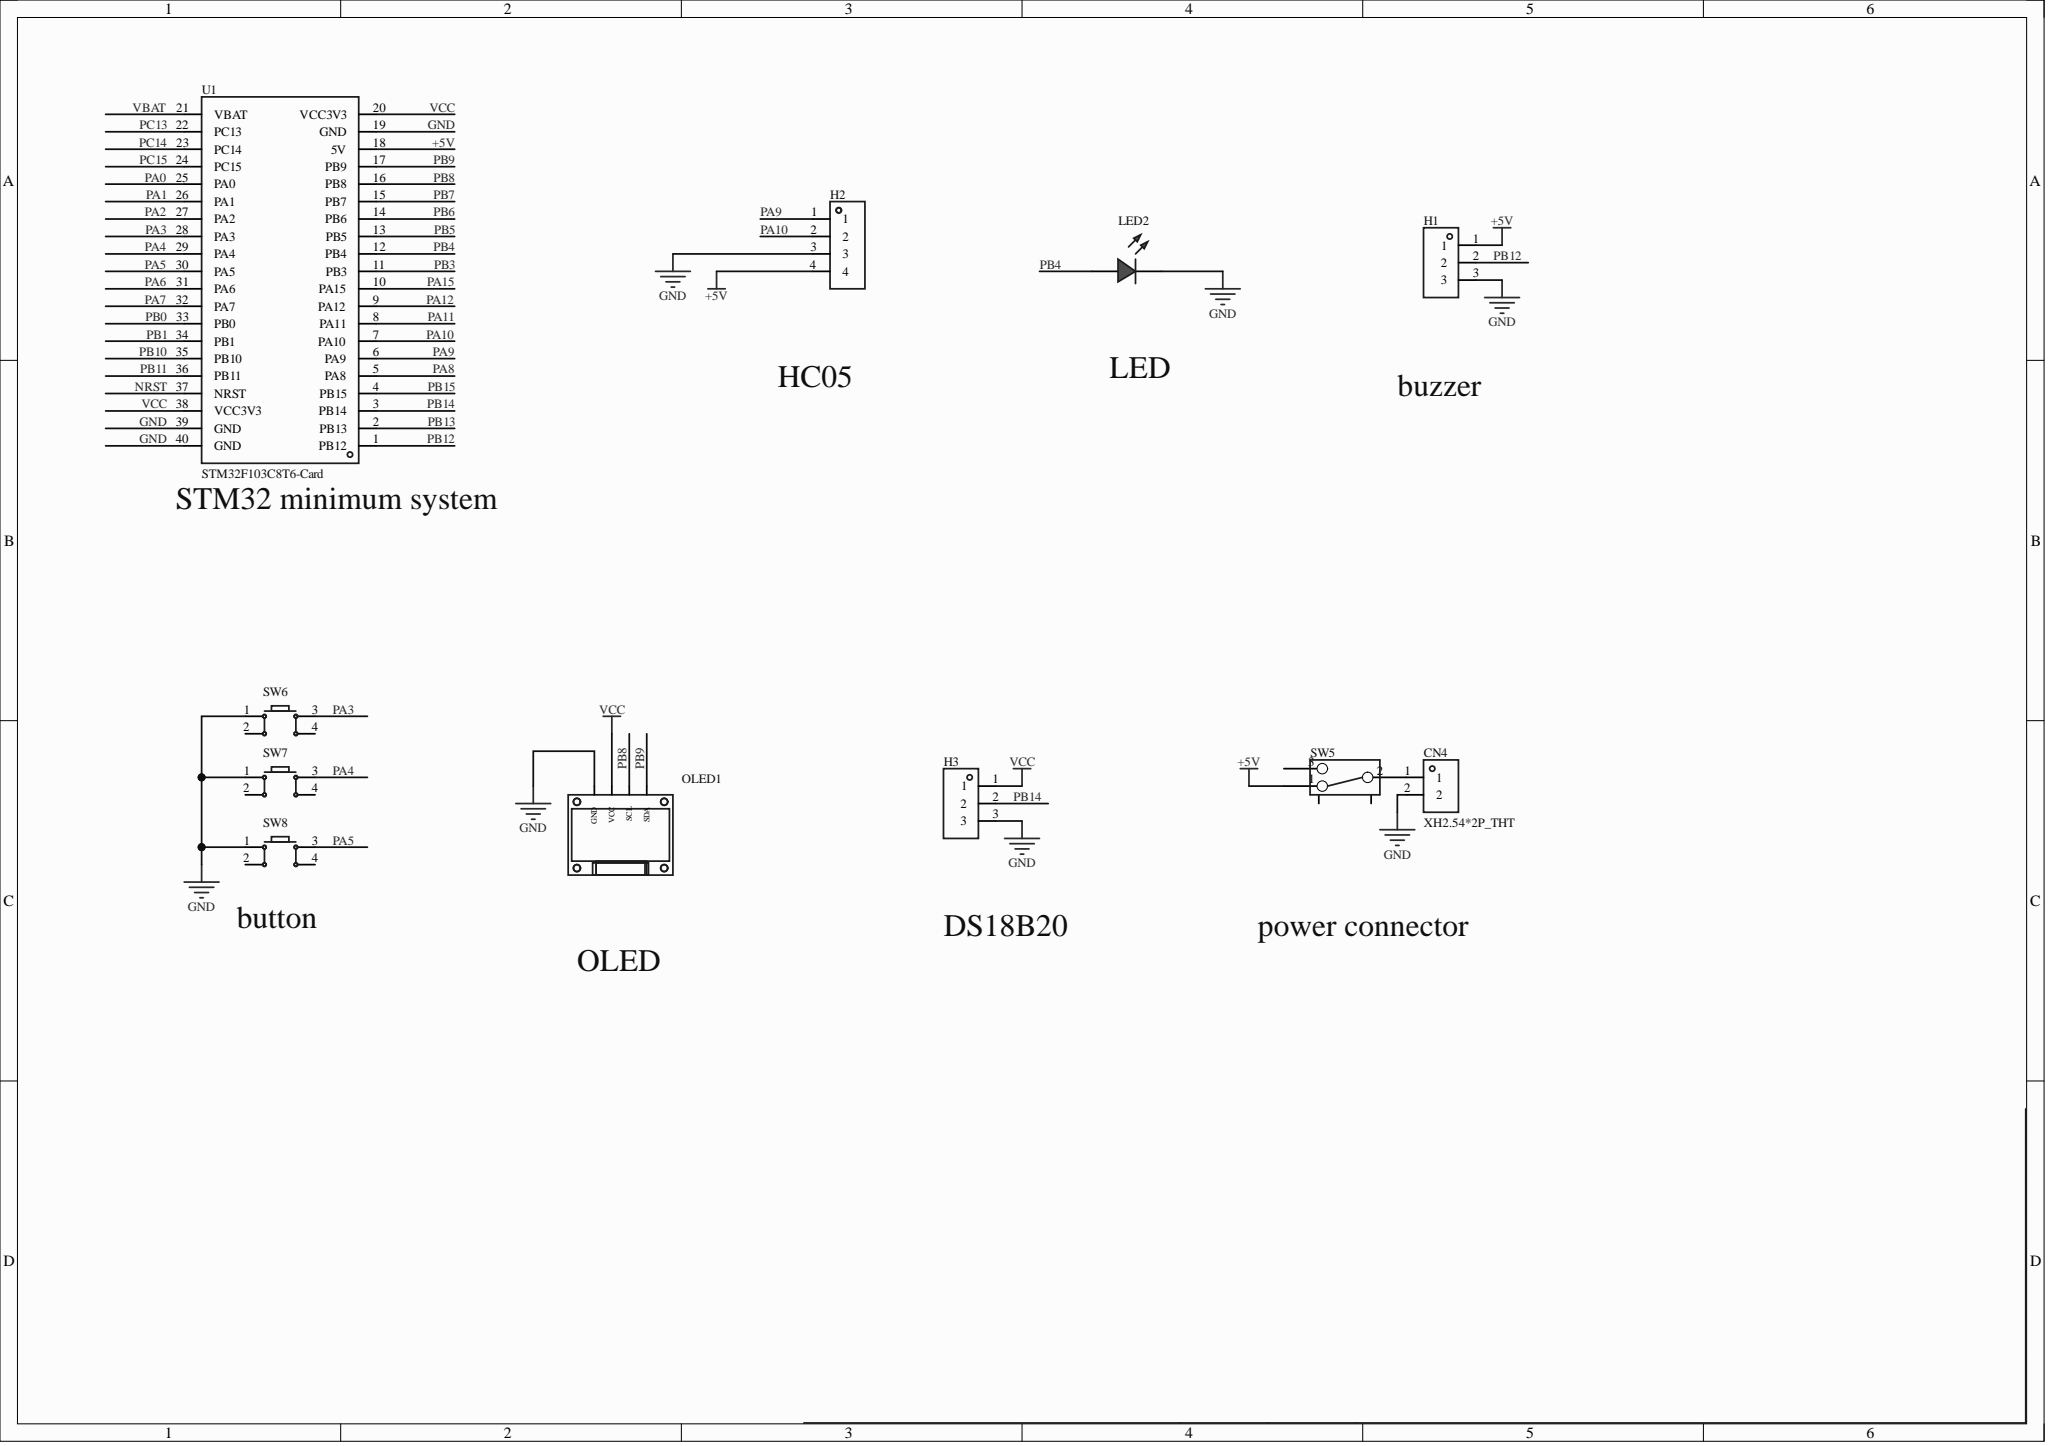Circuit board | Altium Designer | 11 parts | 14 nets
Bill of materials:
Comment,Description,Designator,Footprint,LibRef,Quantity
"XH2.54*2P_THT","","CN4","CONN-TH_2P-P2.50-XH2.54-2P","XH2.54*2P_直插","1"
"","","H1, H3","HDR-TH_3P-P2.54-V-F","HDR-F_2.54_1x3P","2"
"","","H2","HDR-TH_4P-P2.54-V-F","HDR-F_2.54_1x4P","1"
"","","LED2","LED-TH_5mm","LED_TH-R_5mm","1"
"","","OLED1","0.96OLED_4P","0.96OLED模块_4P","1"
"","","SW5","拨动开关","拨动开关_正","1"
"","","SW6, SW7, SW8","SW-TH_4P-L6.0-W6.0-P4.50-LS6.5","Key_TH_6x6x6","3"
"STM32F103C8T6-Card","","U1","CONN-TH_L53.3-W22.9_STM32F103C8T6-CARD","STM32F103C8T6-Card","1"
Netlist (Protel format):
[
CN4
CONN-TH_2P-P2.50-XH2.54-2P
XH2.54*2P_THT



]
[
H1
HDR-TH_3P-P2.54-V-F




]
[
H2
HDR-TH_4P-P2.54-V-F




]
[
H3
HDR-TH_3P-P2.54-V-F




]
[
LED2
LED-TH_5mm




]
[
OLED1
0.96OLED_4P




]
[
SW5
拨动开关




]
[
SW6
SW-TH_4P-L6.0-W6.0-P4.50-LS6.5




]
[
SW7
SW-TH_4P-L6.0-W6.0-P4.50-LS6.5




]
[
SW8
SW-TH_4P-L6.0-W6.0-P4.50-LS6.5




]
[
U1
CONN-TH_L53.3-W22.9_STM32F103C8T6-CARD
STM32F103C8T6-Card



]
(
VCC
H3-1
OLED1-2
U1-20
U1-38
)
(
PB14
H3-2
U1-3
)
(
PB12
H1-2
U1-1
)
(
PB9
OLED1-4
U1-17
)
(
PB8
OLED1-3
U1-16
)
(
PB4
LED2-1
U1-12
)
(
PA10
H2-2
U1-7
)
(
PA9
H2-1
U1-6
)
(
PA5
SW8-3
U1-30
)
(
PA4
SW7-3
U1-29
)
(
PA3
SW6-3
U1-28
)
(
NetCN4_1
CN4-1
SW5-2
)
(
GND
CN4-2
H1-3
H2-3
H3-3
LED2-2
OLED1-1
SW6-1
SW7-1
SW8-1
U1-19
U1-39
U1-40
)
(
+5V
H1-1
H2-4
SW5-1
U1-18
)